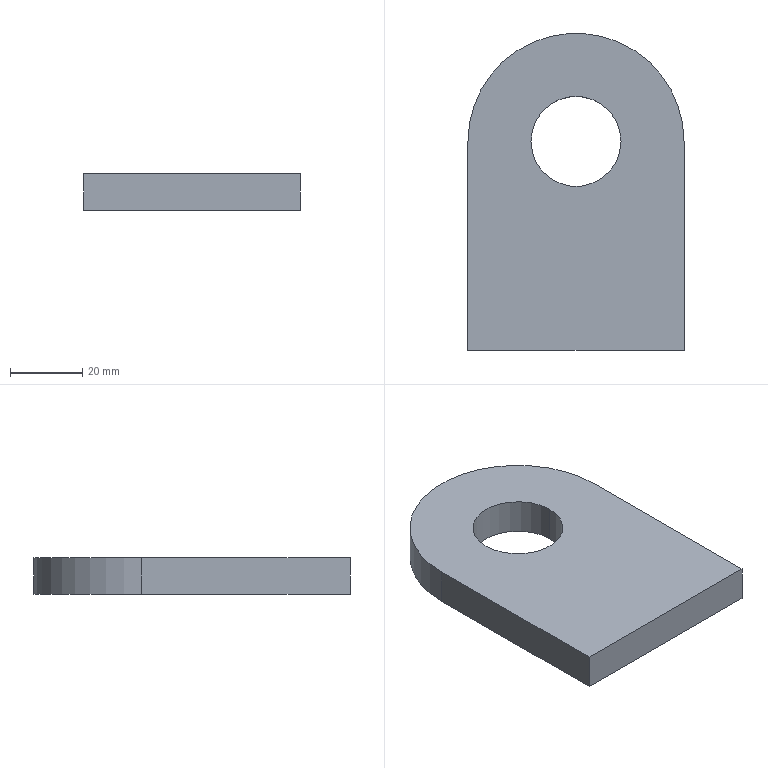Part | SolidWorks | features Extrusion 1 | 1 solid | 8 faces | box 60 x 88 x 10 mm | volume 44028 mm3 | plane 5 | cylinder 3 | commonest cylinder face diameters 25 x2 60 x1
STEP:
#1=CARTESIAN_POINT('',(17.5,58.,10.));
#2=VERTEX_POINT('',#1);
#3=CARTESIAN_POINT('',(42.5,58.,10.));
#4=VERTEX_POINT('',#3);
#5=CARTESIAN_POINT('',(30.,58.,10.));
#6=DIRECTION('',(0.,0.,1.));
#7=DIRECTION('',(1.,0.,0.));
#8=AXIS2_PLACEMENT_3D('',#5,#6,#7);
#9=CIRCLE('',#8,12.5);
#10=EDGE_CURVE('',#2,#4,#9,.T.);
#11=ORIENTED_EDGE('',*,*,#10,.T.);
#12=CARTESIAN_POINT('',(42.5,58.,0.));
#13=VERTEX_POINT('',#12);
#14=CARTESIAN_POINT('',(42.5,58.,10.));
#15=DIRECTION('',(0.,0.,-1.));
#16=VECTOR('',#15,1000.);
#17=LINE('',#14,#16);
#18=EDGE_CURVE('',#4,#13,#17,.T.);
#19=ORIENTED_EDGE('',*,*,#18,.T.);
#20=CARTESIAN_POINT('',(17.5,58.,0.));
#21=VERTEX_POINT('',#20);
#22=CARTESIAN_POINT('',(30.,58.,0.));
#23=DIRECTION('',(0.,0.,1.));
#24=DIRECTION('',(1.,0.,0.));
#25=AXIS2_PLACEMENT_3D('',#22,#23,#24);
#26=CIRCLE('',#25,12.5);
#27=EDGE_CURVE('',#21,#13,#26,.T.);
#28=ORIENTED_EDGE('',*,*,#27,.F.);
#29=CARTESIAN_POINT('',(17.5,58.,10.));
#30=DIRECTION('',(0.,0.,-1.));
#31=VECTOR('',#30,1000.);
#32=LINE('',#29,#31);
#33=EDGE_CURVE('',#2,#21,#32,.T.);
#34=ORIENTED_EDGE('',*,*,#33,.F.);
#35=EDGE_LOOP('',(#11,#19,#28,#34));
#36=FACE_OUTER_BOUND('',#35,.T.);
#37=CARTESIAN_POINT('',(30.,58.,10.));
#38=DIRECTION('',(0.,0.,-1.));
#39=DIRECTION('',(-1.,0.,0.));
#40=AXIS2_PLACEMENT_3D('',#37,#38,#39);
#41=CYLINDRICAL_SURFACE('',#40,12.5);
#42=ADVANCED_FACE('',(#36),#41,.F.);
#43=CARTESIAN_POINT('',(0.,0.,10.));
#44=VERTEX_POINT('',#43);
#45=CARTESIAN_POINT('',(60.,0.,10.));
#46=VERTEX_POINT('',#45);
#47=CARTESIAN_POINT('',(60.,0.,10.));
#48=DIRECTION('',(1.,0.,0.));
#49=VECTOR('',#48,1000.);
#50=LINE('',#47,#49);
#51=EDGE_CURVE('',#44,#46,#50,.T.);
#52=ORIENTED_EDGE('',*,*,#51,.T.);
#53=CARTESIAN_POINT('',(60.,58.,10.));
#54=VERTEX_POINT('',#53);
#55=CARTESIAN_POINT('',(60.,58.,10.));
#56=DIRECTION('',(0.,1.,0.));
#57=VECTOR('',#56,1000.);
#58=LINE('',#55,#57);
#59=EDGE_CURVE('',#46,#54,#58,.T.);
#60=ORIENTED_EDGE('',*,*,#59,.T.);
#61=CARTESIAN_POINT('',(0.,58.,10.));
#62=VERTEX_POINT('',#61);
#63=CARTESIAN_POINT('',(30.,58.,10.));
#64=DIRECTION('',(0.,0.,1.));
#65=DIRECTION('',(-1.,0.,0.));
#66=AXIS2_PLACEMENT_3D('',#63,#64,#65);
#67=CIRCLE('',#66,30.);
#68=EDGE_CURVE('',#54,#62,#67,.T.);
#69=ORIENTED_EDGE('',*,*,#68,.T.);
#70=CARTESIAN_POINT('',(0.,0.,10.));
#71=DIRECTION('',(0.,-1.,0.));
#72=VECTOR('',#71,1000.);
#73=LINE('',#70,#72);
#74=EDGE_CURVE('',#62,#44,#73,.T.);
#75=ORIENTED_EDGE('',*,*,#74,.T.);
#76=EDGE_LOOP('',(#52,#60,#69,#75));
#77=FACE_OUTER_BOUND('',#76,.T.);
#78=ORIENTED_EDGE('',*,*,#10,.F.);
#79=CARTESIAN_POINT('',(30.,58.,10.));
#80=DIRECTION('',(0.,0.,1.));
#81=DIRECTION('',(1.,0.,0.));
#82=AXIS2_PLACEMENT_3D('',#79,#80,#81);
#83=CIRCLE('',#82,12.5);
#84=EDGE_CURVE('',#4,#2,#83,.T.);
#85=ORIENTED_EDGE('',*,*,#84,.F.);
#86=EDGE_LOOP('',(#78,#85));
#87=FACE_BOUND('',#86,.T.);
#88=CARTESIAN_POINT('',(30.,58.,10.));
#89=DIRECTION('',(0.,0.,-1.));
#90=DIRECTION('',(-1.,0.,0.));
#91=AXIS2_PLACEMENT_3D('',#88,#89,#90);
#92=PLANE('',#91);
#93=ADVANCED_FACE('',(#77,#87),#92,.F.);
#94=CARTESIAN_POINT('',(0.,0.,0.));
#95=VERTEX_POINT('',#94);
#96=CARTESIAN_POINT('',(60.,0.,0.));
#97=VERTEX_POINT('',#96);
#98=CARTESIAN_POINT('',(60.,0.,0.));
#99=DIRECTION('',(1.,0.,0.));
#100=VECTOR('',#99,1000.);
#101=LINE('',#98,#100);
#102=EDGE_CURVE('',#95,#97,#101,.T.);
#103=ORIENTED_EDGE('',*,*,#102,.F.);
#104=CARTESIAN_POINT('',(0.,58.,0.));
#105=VERTEX_POINT('',#104);
#106=CARTESIAN_POINT('',(0.,0.,0.));
#107=DIRECTION('',(0.,-1.,0.));
#108=VECTOR('',#107,1000.);
#109=LINE('',#106,#108);
#110=EDGE_CURVE('',#105,#95,#109,.T.);
#111=ORIENTED_EDGE('',*,*,#110,.F.);
#112=CARTESIAN_POINT('',(60.,58.,0.));
#113=VERTEX_POINT('',#112);
#114=CARTESIAN_POINT('',(30.,58.,0.));
#115=DIRECTION('',(0.,0.,1.));
#116=DIRECTION('',(-1.,0.,0.));
#117=AXIS2_PLACEMENT_3D('',#114,#115,#116);
#118=CIRCLE('',#117,30.);
#119=EDGE_CURVE('',#113,#105,#118,.T.);
#120=ORIENTED_EDGE('',*,*,#119,.F.);
#121=CARTESIAN_POINT('',(60.,58.,0.));
#122=DIRECTION('',(0.,1.,0.));
#123=VECTOR('',#122,1000.);
#124=LINE('',#121,#123);
#125=EDGE_CURVE('',#97,#113,#124,.T.);
#126=ORIENTED_EDGE('',*,*,#125,.F.);
#127=EDGE_LOOP('',(#103,#111,#120,#126));
#128=FACE_OUTER_BOUND('',#127,.T.);
#129=ORIENTED_EDGE('',*,*,#27,.T.);
#130=CARTESIAN_POINT('',(30.,58.,0.));
#131=DIRECTION('',(0.,0.,1.));
#132=DIRECTION('',(1.,0.,0.));
#133=AXIS2_PLACEMENT_3D('',#130,#131,#132);
#134=CIRCLE('',#133,12.5);
#135=EDGE_CURVE('',#13,#21,#134,.T.);
#136=ORIENTED_EDGE('',*,*,#135,.T.);
#137=EDGE_LOOP('',(#129,#136));
#138=FACE_BOUND('',#137,.T.);
#139=CARTESIAN_POINT('',(30.,58.,0.));
#140=DIRECTION('',(0.,0.,-1.));
#141=DIRECTION('',(-1.,0.,0.));
#142=AXIS2_PLACEMENT_3D('',#139,#140,#141);
#143=PLANE('',#142);
#144=ADVANCED_FACE('',(#128,#138),#143,.T.);
#145=ORIENTED_EDGE('',*,*,#102,.T.);
#146=CARTESIAN_POINT('',(60.,0.,10.));
#147=DIRECTION('',(0.,0.,-1.));
#148=VECTOR('',#147,1000.);
#149=LINE('',#146,#148);
#150=EDGE_CURVE('',#46,#97,#149,.T.);
#151=ORIENTED_EDGE('',*,*,#150,.F.);
#152=ORIENTED_EDGE('',*,*,#51,.F.);
#153=CARTESIAN_POINT('',(0.,0.,10.));
#154=DIRECTION('',(0.,0.,-1.));
#155=VECTOR('',#154,1000.);
#156=LINE('',#153,#155);
#157=EDGE_CURVE('',#44,#95,#156,.T.);
#158=ORIENTED_EDGE('',*,*,#157,.T.);
#159=EDGE_LOOP('',(#145,#151,#152,#158));
#160=FACE_OUTER_BOUND('',#159,.T.);
#161=CARTESIAN_POINT('',(60.,0.,10.));
#162=DIRECTION('',(0.,1.,0.));
#163=DIRECTION('',(0.,0.,1.));
#164=AXIS2_PLACEMENT_3D('',#161,#162,#163);
#165=PLANE('',#164);
#166=ADVANCED_FACE('',(#160),#165,.F.);
#167=ORIENTED_EDGE('',*,*,#125,.T.);
#168=CARTESIAN_POINT('',(60.,58.,10.));
#169=DIRECTION('',(0.,0.,-1.));
#170=VECTOR('',#169,1000.);
#171=LINE('',#168,#170);
#172=EDGE_CURVE('',#54,#113,#171,.T.);
#173=ORIENTED_EDGE('',*,*,#172,.F.);
#174=ORIENTED_EDGE('',*,*,#59,.F.);
#175=ORIENTED_EDGE('',*,*,#150,.T.);
#176=EDGE_LOOP('',(#167,#173,#174,#175));
#177=FACE_OUTER_BOUND('',#176,.T.);
#178=CARTESIAN_POINT('',(60.,58.,10.));
#179=DIRECTION('',(-1.,0.,0.));
#180=DIRECTION('',(0.,0.,1.));
#181=AXIS2_PLACEMENT_3D('',#178,#179,#180);
#182=PLANE('',#181);
#183=ADVANCED_FACE('',(#177),#182,.F.);
#184=ORIENTED_EDGE('',*,*,#119,.T.);
#185=CARTESIAN_POINT('',(0.,58.,10.));
#186=DIRECTION('',(0.,0.,-1.));
#187=VECTOR('',#186,1000.);
#188=LINE('',#185,#187);
#189=EDGE_CURVE('',#62,#105,#188,.T.);
#190=ORIENTED_EDGE('',*,*,#189,.F.);
#191=ORIENTED_EDGE('',*,*,#68,.F.);
#192=ORIENTED_EDGE('',*,*,#172,.T.);
#193=EDGE_LOOP('',(#184,#190,#191,#192));
#194=FACE_OUTER_BOUND('',#193,.T.);
#195=CARTESIAN_POINT('',(30.,58.,10.));
#196=DIRECTION('',(0.,0.,-1.));
#197=DIRECTION('',(-1.,0.,0.));
#198=AXIS2_PLACEMENT_3D('',#195,#196,#197);
#199=CYLINDRICAL_SURFACE('',#198,30.);
#200=ADVANCED_FACE('',(#194),#199,.T.);
#201=ORIENTED_EDGE('',*,*,#110,.T.);
#202=ORIENTED_EDGE('',*,*,#157,.F.);
#203=ORIENTED_EDGE('',*,*,#74,.F.);
#204=ORIENTED_EDGE('',*,*,#189,.T.);
#205=EDGE_LOOP('',(#201,#202,#203,#204));
#206=FACE_OUTER_BOUND('',#205,.T.);
#207=CARTESIAN_POINT('',(0.,0.,10.));
#208=DIRECTION('',(1.,0.,0.));
#209=DIRECTION('',(0.,0.,-1.));
#210=AXIS2_PLACEMENT_3D('',#207,#208,#209);
#211=PLANE('',#210);
#212=ADVANCED_FACE('',(#206),#211,.F.);
#213=ORIENTED_EDGE('',*,*,#18,.F.);
#214=ORIENTED_EDGE('',*,*,#84,.T.);
#215=ORIENTED_EDGE('',*,*,#33,.T.);
#216=ORIENTED_EDGE('',*,*,#135,.F.);
#217=EDGE_LOOP('',(#213,#214,#215,#216));
#218=FACE_OUTER_BOUND('',#217,.T.);
#219=CARTESIAN_POINT('',(30.,58.,10.));
#220=DIRECTION('',(0.,0.,-1.));
#221=DIRECTION('',(-1.,0.,0.));
#222=AXIS2_PLACEMENT_3D('',#219,#220,#221);
#223=CYLINDRICAL_SURFACE('',#222,12.5);
#224=ADVANCED_FACE('',(#218),#223,.F.);
#225=CLOSED_SHELL('',(#42,#93,#144,#166,#183,#200,#212,#224));
#226=MANIFOLD_SOLID_BREP('',#225);
#227=CARTESIAN_POINT('',(0.,0.,0.));
#228=DIRECTION('',(0.,0.,1.));
#229=DIRECTION('',(1.,0.,0.));
#230=AXIS2_PLACEMENT_3D('',#227,#228,#229);
#231=(LENGTH_UNIT()NAMED_UNIT(*)SI_UNIT(.MILLI.,.METRE.));
#232=UNCERTAINTY_MEASURE_WITH_UNIT(LENGTH_MEASURE(0.00001),#231,'','');
#233=(NAMED_UNIT(*)PLANE_ANGLE_UNIT()SI_UNIT($,.RADIAN.));
#234=(NAMED_UNIT(*)SI_UNIT($,.STERADIAN.)SOLID_ANGLE_UNIT());
#235=(GEOMETRIC_REPRESENTATION_CONTEXT(3)GLOBAL_UNCERTAINTY_ASSIGNED_CONTEXT((#232))GLOBAL_UNIT_ASSIGNED_CONTEXT((#231,#233,#234))REPRESENTATION_CONTEXT('',''));
#236=ADVANCED_BREP_SHAPE_REPRESENTATION('',(#226,#230),#235);